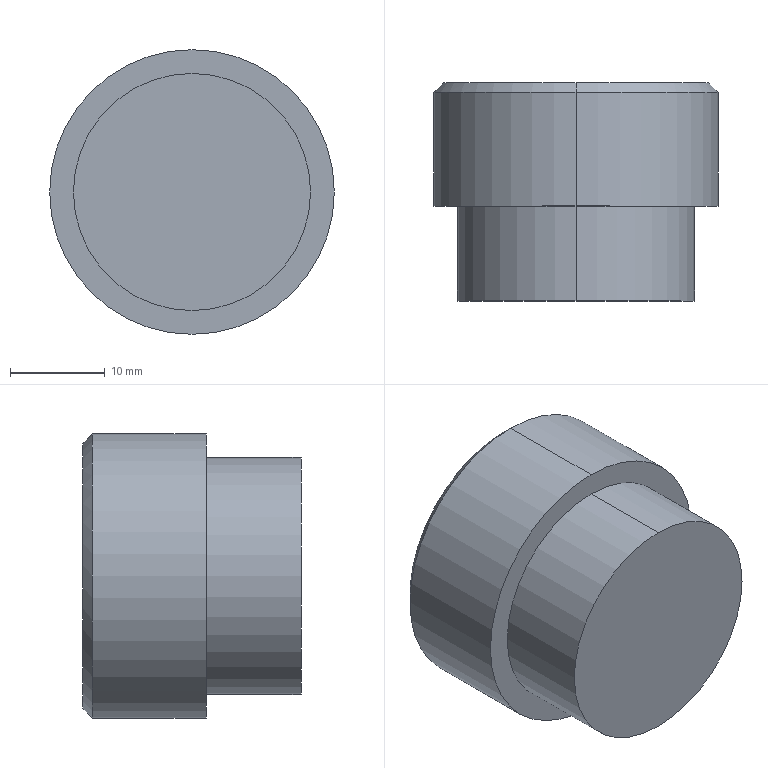Part | SolidWorks | features Chamfer 1, Extrusion 1, ICE 1 | 1 solid | 9 faces | box 30 x 23 x 30 mm | volume 14052 mm3 | cylinder 4 | plane 3 | cone 2 | commonest cylinder face diameters 25 x2 30 x2
STEP:
#1=CARTESIAN_POINT('',(0.,13.,14.));
#2=VERTEX_POINT('',#1);
#3=CARTESIAN_POINT('',(0.,13.,-14.));
#4=VERTEX_POINT('',#3);
#5=CARTESIAN_POINT('',(0.,13.,0.));
#6=DIRECTION('',(0.,1.,0.));
#7=DIRECTION('',(0.,0.,1.));
#8=AXIS2_PLACEMENT_3D('',#5,#6,#7);
#9=CIRCLE('',#8,14.);
#10=EDGE_CURVE('',#2,#4,#9,.T.);
#11=ORIENTED_EDGE('',*,*,#10,.F.);
#12=CARTESIAN_POINT('',(0.,12.,15.));
#13=VERTEX_POINT('',#12);
#14=CARTESIAN_POINT('',(0.,13.,14.));
#15=DIRECTION('',(0.,-0.7071,0.7071));
#16=VECTOR('',#15,1000.);
#17=LINE('',#14,#16);
#18=EDGE_CURVE('',#2,#13,#17,.T.);
#19=ORIENTED_EDGE('',*,*,#18,.T.);
#20=CARTESIAN_POINT('',(0.,12.,-15.));
#21=VERTEX_POINT('',#20);
#22=CARTESIAN_POINT('',(0.,12.,0.));
#23=DIRECTION('',(0.,-1.,0.));
#24=DIRECTION('',(0.,0.,1.));
#25=AXIS2_PLACEMENT_3D('',#22,#23,#24);
#26=CIRCLE('',#25,15.);
#27=EDGE_CURVE('',#21,#13,#26,.T.);
#28=ORIENTED_EDGE('',*,*,#27,.F.);
#29=CARTESIAN_POINT('',(0.,13.,-14.));
#30=DIRECTION('',(0.,-0.7071,-0.7071));
#31=VECTOR('',#30,1000.);
#32=LINE('',#29,#31);
#33=EDGE_CURVE('',#4,#21,#32,.T.);
#34=ORIENTED_EDGE('',*,*,#33,.F.);
#35=EDGE_LOOP('',(#11,#19,#28,#34));
#36=FACE_OUTER_BOUND('',#35,.T.);
#37=CARTESIAN_POINT('',(0.,13.,0.));
#38=DIRECTION('',(0.,-1.,0.));
#39=DIRECTION('',(0.,0.,-1.));
#40=AXIS2_PLACEMENT_3D('',#37,#38,#39);
#41=CONICAL_SURFACE('',#40,14.,0.7854);
#42=ADVANCED_FACE('',(#36),#41,.T.);
#43=CARTESIAN_POINT('',(0.,-10.,-12.5));
#44=VERTEX_POINT('',#43);
#45=CARTESIAN_POINT('',(0.,-10.,12.5));
#46=VERTEX_POINT('',#45);
#47=CARTESIAN_POINT('',(0.,-10.,0.));
#48=DIRECTION('',(0.,-1.,0.));
#49=DIRECTION('',(0.,0.,-1.));
#50=AXIS2_PLACEMENT_3D('',#47,#48,#49);
#51=CIRCLE('',#50,12.5);
#52=EDGE_CURVE('',#44,#46,#51,.T.);
#53=ORIENTED_EDGE('',*,*,#52,.F.);
#54=CARTESIAN_POINT('',(0.,0.,-12.5));
#55=VERTEX_POINT('',#54);
#56=CARTESIAN_POINT('',(0.,-10.,-12.5));
#57=DIRECTION('',(0.,1.,0.));
#58=VECTOR('',#57,1000.);
#59=LINE('',#56,#58);
#60=EDGE_CURVE('',#44,#55,#59,.T.);
#61=ORIENTED_EDGE('',*,*,#60,.T.);
#62=CARTESIAN_POINT('',(0.,0.,12.5));
#63=VERTEX_POINT('',#62);
#64=CARTESIAN_POINT('',(0.,0.,0.));
#65=DIRECTION('',(0.,-1.,0.));
#66=DIRECTION('',(0.,0.,-1.));
#67=AXIS2_PLACEMENT_3D('',#64,#65,#66);
#68=CIRCLE('',#67,12.5);
#69=EDGE_CURVE('',#55,#63,#68,.T.);
#70=ORIENTED_EDGE('',*,*,#69,.T.);
#71=CARTESIAN_POINT('',(0.,-10.,12.5));
#72=DIRECTION('',(0.,1.,0.));
#73=VECTOR('',#72,1000.);
#74=LINE('',#71,#73);
#75=EDGE_CURVE('',#46,#63,#74,.T.);
#76=ORIENTED_EDGE('',*,*,#75,.F.);
#77=EDGE_LOOP('',(#53,#61,#70,#76));
#78=FACE_OUTER_BOUND('',#77,.T.);
#79=CARTESIAN_POINT('',(0.,-10.,0.));
#80=DIRECTION('',(0.,1.,0.));
#81=DIRECTION('',(0.,0.,1.));
#82=AXIS2_PLACEMENT_3D('',#79,#80,#81);
#83=CYLINDRICAL_SURFACE('',#82,12.5);
#84=ADVANCED_FACE('',(#78),#83,.T.);
#85=ORIENTED_EDGE('',*,*,#27,.T.);
#86=CARTESIAN_POINT('',(0.,0.,15.));
#87=VERTEX_POINT('',#86);
#88=CARTESIAN_POINT('',(0.,13.,15.));
#89=DIRECTION('',(0.,-1.,0.));
#90=VECTOR('',#89,1000.);
#91=LINE('',#88,#90);
#92=EDGE_CURVE('',#13,#87,#91,.T.);
#93=ORIENTED_EDGE('',*,*,#92,.T.);
#94=CARTESIAN_POINT('',(0.,0.,-15.));
#95=VERTEX_POINT('',#94);
#96=CARTESIAN_POINT('',(0.,0.,0.));
#97=DIRECTION('',(0.,1.,0.));
#98=DIRECTION('',(0.,0.,1.));
#99=AXIS2_PLACEMENT_3D('',#96,#97,#98);
#100=CIRCLE('',#99,15.);
#101=EDGE_CURVE('',#87,#95,#100,.T.);
#102=ORIENTED_EDGE('',*,*,#101,.T.);
#103=CARTESIAN_POINT('',(0.,13.,-15.));
#104=DIRECTION('',(0.,-1.,0.));
#105=VECTOR('',#104,1000.);
#106=LINE('',#103,#105);
#107=EDGE_CURVE('',#21,#95,#106,.T.);
#108=ORIENTED_EDGE('',*,*,#107,.F.);
#109=EDGE_LOOP('',(#85,#93,#102,#108));
#110=FACE_OUTER_BOUND('',#109,.T.);
#111=CARTESIAN_POINT('',(0.,13.,0.));
#112=DIRECTION('',(0.,-1.,0.));
#113=DIRECTION('',(0.,0.,-1.));
#114=AXIS2_PLACEMENT_3D('',#111,#112,#113);
#115=CYLINDRICAL_SURFACE('',#114,15.);
#116=ADVANCED_FACE('',(#110),#115,.T.);
#117=ORIENTED_EDGE('',*,*,#92,.F.);
#118=CARTESIAN_POINT('',(0.,12.,0.));
#119=DIRECTION('',(0.,-1.,0.));
#120=DIRECTION('',(0.,0.,1.));
#121=AXIS2_PLACEMENT_3D('',#118,#119,#120);
#122=CIRCLE('',#121,15.);
#123=EDGE_CURVE('',#13,#21,#122,.T.);
#124=ORIENTED_EDGE('',*,*,#123,.T.);
#125=ORIENTED_EDGE('',*,*,#107,.T.);
#126=CARTESIAN_POINT('',(0.,0.,0.));
#127=DIRECTION('',(0.,1.,0.));
#128=DIRECTION('',(0.,0.,1.));
#129=AXIS2_PLACEMENT_3D('',#126,#127,#128);
#130=CIRCLE('',#129,15.);
#131=EDGE_CURVE('',#95,#87,#130,.T.);
#132=ORIENTED_EDGE('',*,*,#131,.T.);
#133=EDGE_LOOP('',(#117,#124,#125,#132));
#134=FACE_OUTER_BOUND('',#133,.T.);
#135=CARTESIAN_POINT('',(0.,13.,0.));
#136=DIRECTION('',(0.,-1.,0.));
#137=DIRECTION('',(0.,0.,-1.));
#138=AXIS2_PLACEMENT_3D('',#135,#136,#137);
#139=CYLINDRICAL_SURFACE('',#138,15.);
#140=ADVANCED_FACE('',(#134),#139,.T.);
#141=CARTESIAN_POINT('',(0.,13.,0.));
#142=DIRECTION('',(0.,1.,0.));
#143=DIRECTION('',(0.,0.,1.));
#144=AXIS2_PLACEMENT_3D('',#141,#142,#143);
#145=CIRCLE('',#144,14.);
#146=EDGE_CURVE('',#4,#2,#145,.T.);
#147=ORIENTED_EDGE('',*,*,#146,.T.);
#148=ORIENTED_EDGE('',*,*,#10,.T.);
#149=EDGE_LOOP('',(#147,#148));
#150=FACE_OUTER_BOUND('',#149,.T.);
#151=CARTESIAN_POINT('',(0.,13.,0.));
#152=DIRECTION('',(0.,1.,0.));
#153=DIRECTION('',(0.,0.,1.));
#154=AXIS2_PLACEMENT_3D('',#151,#152,#153);
#155=PLANE('',#154);
#156=ADVANCED_FACE('',(#150),#155,.T.);
#157=CARTESIAN_POINT('',(0.,0.,0.));
#158=DIRECTION('',(0.,-1.,0.));
#159=DIRECTION('',(0.,0.,-1.));
#160=AXIS2_PLACEMENT_3D('',#157,#158,#159);
#161=CIRCLE('',#160,12.5);
#162=EDGE_CURVE('',#63,#55,#161,.T.);
#163=ORIENTED_EDGE('',*,*,#162,.F.);
#164=ORIENTED_EDGE('',*,*,#69,.F.);
#165=EDGE_LOOP('',(#163,#164));
#166=FACE_BOUND('',#165,.T.);
#167=ORIENTED_EDGE('',*,*,#131,.F.);
#168=ORIENTED_EDGE('',*,*,#101,.F.);
#169=EDGE_LOOP('',(#167,#168));
#170=FACE_OUTER_BOUND('',#169,.T.);
#171=CARTESIAN_POINT('',(0.,0.,0.));
#172=DIRECTION('',(0.,1.,0.));
#173=DIRECTION('',(0.,0.,1.));
#174=AXIS2_PLACEMENT_3D('',#171,#172,#173);
#175=PLANE('',#174);
#176=ADVANCED_FACE('',(#166,#170),#175,.F.);
#177=ORIENTED_EDGE('',*,*,#60,.F.);
#178=CARTESIAN_POINT('',(0.,-10.,0.));
#179=DIRECTION('',(0.,-1.,0.));
#180=DIRECTION('',(0.,0.,-1.));
#181=AXIS2_PLACEMENT_3D('',#178,#179,#180);
#182=CIRCLE('',#181,12.5);
#183=EDGE_CURVE('',#46,#44,#182,.T.);
#184=ORIENTED_EDGE('',*,*,#183,.F.);
#185=ORIENTED_EDGE('',*,*,#75,.T.);
#186=ORIENTED_EDGE('',*,*,#162,.T.);
#187=EDGE_LOOP('',(#177,#184,#185,#186));
#188=FACE_OUTER_BOUND('',#187,.T.);
#189=CARTESIAN_POINT('',(0.,-10.,0.));
#190=DIRECTION('',(0.,1.,0.));
#191=DIRECTION('',(0.,0.,1.));
#192=AXIS2_PLACEMENT_3D('',#189,#190,#191);
#193=CYLINDRICAL_SURFACE('',#192,12.5);
#194=ADVANCED_FACE('',(#188),#193,.T.);
#195=ORIENTED_EDGE('',*,*,#183,.T.);
#196=ORIENTED_EDGE('',*,*,#52,.T.);
#197=EDGE_LOOP('',(#195,#196));
#198=FACE_OUTER_BOUND('',#197,.T.);
#199=CARTESIAN_POINT('',(0.,-10.,0.));
#200=DIRECTION('',(0.,-1.,0.));
#201=DIRECTION('',(0.,0.,-1.));
#202=AXIS2_PLACEMENT_3D('',#199,#200,#201);
#203=PLANE('',#202);
#204=ADVANCED_FACE('',(#198),#203,.T.);
#205=ORIENTED_EDGE('',*,*,#18,.F.);
#206=ORIENTED_EDGE('',*,*,#146,.F.);
#207=ORIENTED_EDGE('',*,*,#33,.T.);
#208=ORIENTED_EDGE('',*,*,#123,.F.);
#209=EDGE_LOOP('',(#205,#206,#207,#208));
#210=FACE_OUTER_BOUND('',#209,.T.);
#211=CARTESIAN_POINT('',(0.,13.,0.));
#212=DIRECTION('',(0.,-1.,0.));
#213=DIRECTION('',(0.,0.,-1.));
#214=AXIS2_PLACEMENT_3D('',#211,#212,#213);
#215=CONICAL_SURFACE('',#214,14.,0.7854);
#216=ADVANCED_FACE('',(#210),#215,.T.);
#217=CLOSED_SHELL('',(#42,#84,#116,#140,#156,#176,#194,#204,#216));
#218=MANIFOLD_SOLID_BREP('',#217);
#219=CARTESIAN_POINT('',(0.,0.,0.));
#220=DIRECTION('',(0.,0.,1.));
#221=DIRECTION('',(1.,0.,0.));
#222=AXIS2_PLACEMENT_3D('',#219,#220,#221);
#223=(LENGTH_UNIT()NAMED_UNIT(*)SI_UNIT(.MILLI.,.METRE.));
#224=UNCERTAINTY_MEASURE_WITH_UNIT(LENGTH_MEASURE(0.00001),#223,'','');
#225=(NAMED_UNIT(*)PLANE_ANGLE_UNIT()SI_UNIT($,.RADIAN.));
#226=(NAMED_UNIT(*)SI_UNIT($,.STERADIAN.)SOLID_ANGLE_UNIT());
#227=(GEOMETRIC_REPRESENTATION_CONTEXT(3)GLOBAL_UNCERTAINTY_ASSIGNED_CONTEXT((#224))GLOBAL_UNIT_ASSIGNED_CONTEXT((#223,#225,#226))REPRESENTATION_CONTEXT('',''));
#228=ADVANCED_BREP_SHAPE_REPRESENTATION('',(#218,#222),#227);